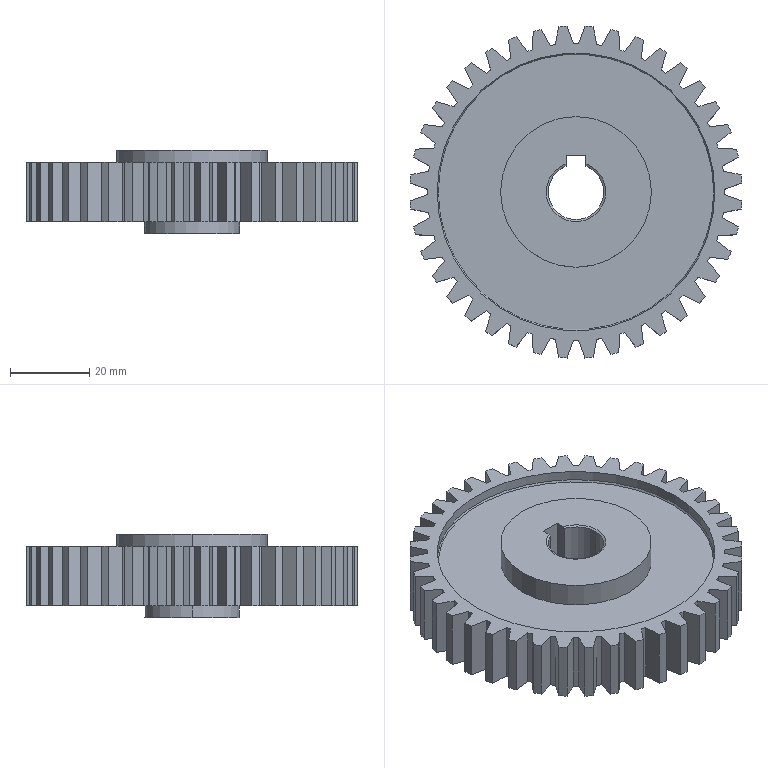Part | SolidWorks | features ICE 5, Chamfer 2, CirPattern 1, Extrusion 1 | 1 solid | 185 faces | box 83.67 x 83.67 x 21 mm | volume 68213 mm3 | plane 128 | cylinder 49 | cone 8 | commonest cylinder face diameters 83.79 x40 14 x3 24 x2 38 x2 70 x2